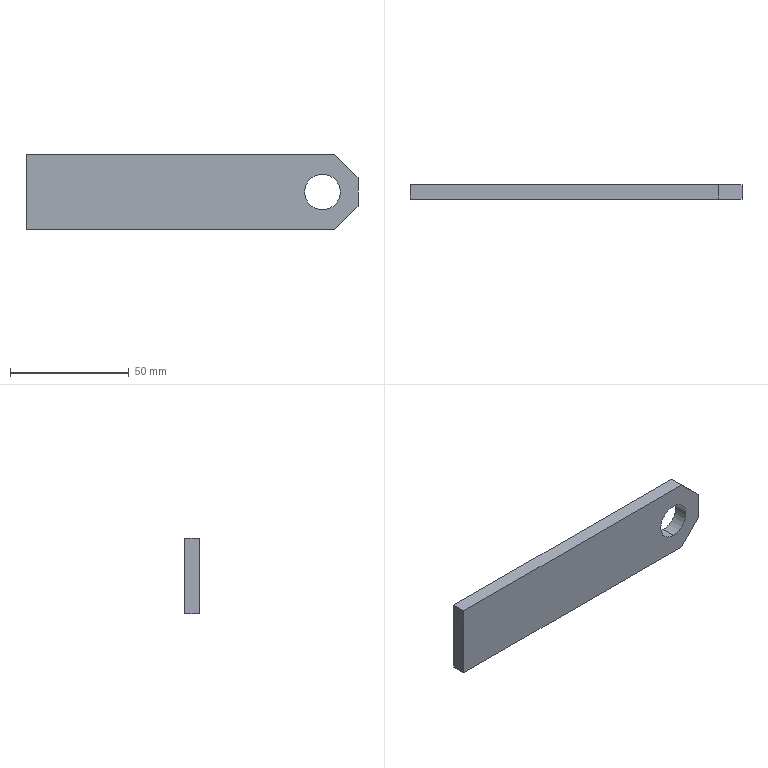Part | SolidWorks | features FlatPattern 1, SMBaseFlange 1, SheetMetal 1 | 1 solid | 10 faces | box 140 x 6 x 32 mm | volume 25220 mm3 | plane 8 | cylinder 2 | commonest cylinder face diameters 15 x2
STEP:
#1=CARTESIAN_POINT('',(125.,-6.,8.5));
#2=VERTEX_POINT('',#1);
#3=CARTESIAN_POINT('',(125.,-6.,23.5));
#4=VERTEX_POINT('',#3);
#5=CARTESIAN_POINT('',(125.,-6.,16.));
#6=DIRECTION('',(0.,1.,0.));
#7=DIRECTION('',(0.,0.,1.));
#8=AXIS2_PLACEMENT_3D('',#5,#6,#7);
#9=CIRCLE('',#8,7.5);
#10=EDGE_CURVE('',#2,#4,#9,.T.);
#11=ORIENTED_EDGE('',*,*,#10,.F.);
#12=CARTESIAN_POINT('',(125.,0.,8.5));
#13=VERTEX_POINT('',#12);
#14=CARTESIAN_POINT('',(125.,-6.,8.5));
#15=DIRECTION('',(0.,1.,0.));
#16=VECTOR('',#15,1000.);
#17=LINE('',#14,#16);
#18=EDGE_CURVE('',#2,#13,#17,.T.);
#19=ORIENTED_EDGE('',*,*,#18,.T.);
#20=CARTESIAN_POINT('',(125.,0.,23.5));
#21=VERTEX_POINT('',#20);
#22=CARTESIAN_POINT('',(125.,0.,16.));
#23=DIRECTION('',(0.,1.,0.));
#24=DIRECTION('',(0.,0.,1.));
#25=AXIS2_PLACEMENT_3D('',#22,#23,#24);
#26=CIRCLE('',#25,7.5);
#27=EDGE_CURVE('',#13,#21,#26,.T.);
#28=ORIENTED_EDGE('',*,*,#27,.T.);
#29=CARTESIAN_POINT('',(125.,-6.,23.5));
#30=DIRECTION('',(0.,1.,0.));
#31=VECTOR('',#30,1000.);
#32=LINE('',#29,#31);
#33=EDGE_CURVE('',#4,#21,#32,.T.);
#34=ORIENTED_EDGE('',*,*,#33,.F.);
#35=EDGE_LOOP('',(#11,#19,#28,#34));
#36=FACE_OUTER_BOUND('',#35,.T.);
#37=CARTESIAN_POINT('',(125.,-6.,16.));
#38=DIRECTION('',(0.,1.,0.));
#39=DIRECTION('',(0.,0.,1.));
#40=AXIS2_PLACEMENT_3D('',#37,#38,#39);
#41=CYLINDRICAL_SURFACE('',#40,7.5);
#42=ADVANCED_FACE('',(#36),#41,.F.);
#43=CARTESIAN_POINT('',(0.,0.,0.));
#44=VERTEX_POINT('',#43);
#45=CARTESIAN_POINT('',(0.,0.,32.));
#46=VERTEX_POINT('',#45);
#47=CARTESIAN_POINT('',(0.,0.,0.));
#48=DIRECTION('',(0.,0.,1.));
#49=VECTOR('',#48,1000.);
#50=LINE('',#47,#49);
#51=EDGE_CURVE('',#44,#46,#50,.T.);
#52=ORIENTED_EDGE('',*,*,#51,.F.);
#53=CARTESIAN_POINT('',(0.,-6.,0.));
#54=VERTEX_POINT('',#53);
#55=CARTESIAN_POINT('',(0.,-6.,0.));
#56=DIRECTION('',(0.,1.,0.));
#57=VECTOR('',#56,1000.);
#58=LINE('',#55,#57);
#59=EDGE_CURVE('',#54,#44,#58,.T.);
#60=ORIENTED_EDGE('',*,*,#59,.F.);
#61=CARTESIAN_POINT('',(0.,-6.,32.));
#62=VERTEX_POINT('',#61);
#63=CARTESIAN_POINT('',(0.,-6.,0.));
#64=DIRECTION('',(0.,0.,1.));
#65=VECTOR('',#64,1000.);
#66=LINE('',#63,#65);
#67=EDGE_CURVE('',#54,#62,#66,.T.);
#68=ORIENTED_EDGE('',*,*,#67,.T.);
#69=CARTESIAN_POINT('',(0.,-6.,32.));
#70=DIRECTION('',(0.,1.,0.));
#71=VECTOR('',#70,1000.);
#72=LINE('',#69,#71);
#73=EDGE_CURVE('',#62,#46,#72,.T.);
#74=ORIENTED_EDGE('',*,*,#73,.T.);
#75=EDGE_LOOP('',(#52,#60,#68,#74));
#76=FACE_OUTER_BOUND('',#75,.T.);
#77=CARTESIAN_POINT('',(0.,-6.,0.));
#78=DIRECTION('',(-1.,0.,0.));
#79=DIRECTION('',(0.,0.,1.));
#80=AXIS2_PLACEMENT_3D('',#77,#78,#79);
#81=PLANE('',#80);
#82=ADVANCED_FACE('',(#76),#81,.T.);
#83=CARTESIAN_POINT('',(130.,0.,0.));
#84=VERTEX_POINT('',#83);
#85=CARTESIAN_POINT('',(0.,0.,0.));
#86=DIRECTION('',(-1.,0.,0.));
#87=VECTOR('',#86,1000.);
#88=LINE('',#85,#87);
#89=EDGE_CURVE('',#84,#44,#88,.T.);
#90=ORIENTED_EDGE('',*,*,#89,.F.);
#91=CARTESIAN_POINT('',(130.,-6.,0.));
#92=VERTEX_POINT('',#91);
#93=CARTESIAN_POINT('',(130.,-6.,0.));
#94=DIRECTION('',(0.,1.,0.));
#95=VECTOR('',#94,1000.);
#96=LINE('',#93,#95);
#97=EDGE_CURVE('',#92,#84,#96,.T.);
#98=ORIENTED_EDGE('',*,*,#97,.F.);
#99=CARTESIAN_POINT('',(0.,-6.,0.));
#100=DIRECTION('',(-1.,0.,0.));
#101=VECTOR('',#100,1000.);
#102=LINE('',#99,#101);
#103=EDGE_CURVE('',#92,#54,#102,.T.);
#104=ORIENTED_EDGE('',*,*,#103,.T.);
#105=ORIENTED_EDGE('',*,*,#59,.T.);
#106=EDGE_LOOP('',(#90,#98,#104,#105));
#107=FACE_OUTER_BOUND('',#106,.T.);
#108=CARTESIAN_POINT('',(0.,-6.,0.));
#109=DIRECTION('',(0.,0.,-1.));
#110=DIRECTION('',(-1.,0.,0.));
#111=AXIS2_PLACEMENT_3D('',#108,#109,#110);
#112=PLANE('',#111);
#113=ADVANCED_FACE('',(#107),#112,.T.);
#114=CARTESIAN_POINT('',(140.,0.,10.));
#115=VERTEX_POINT('',#114);
#116=CARTESIAN_POINT('',(130.,0.,0.));
#117=DIRECTION('',(-0.7071,0.,-0.7071));
#118=VECTOR('',#117,1000.);
#119=LINE('',#116,#118);
#120=EDGE_CURVE('',#115,#84,#119,.T.);
#121=ORIENTED_EDGE('',*,*,#120,.F.);
#122=CARTESIAN_POINT('',(140.,-6.,10.));
#123=VERTEX_POINT('',#122);
#124=CARTESIAN_POINT('',(140.,-6.,10.));
#125=DIRECTION('',(0.,1.,0.));
#126=VECTOR('',#125,1000.);
#127=LINE('',#124,#126);
#128=EDGE_CURVE('',#123,#115,#127,.T.);
#129=ORIENTED_EDGE('',*,*,#128,.F.);
#130=CARTESIAN_POINT('',(130.,-6.,0.));
#131=DIRECTION('',(-0.7071,0.,-0.7071));
#132=VECTOR('',#131,1000.);
#133=LINE('',#130,#132);
#134=EDGE_CURVE('',#123,#92,#133,.T.);
#135=ORIENTED_EDGE('',*,*,#134,.T.);
#136=ORIENTED_EDGE('',*,*,#97,.T.);
#137=EDGE_LOOP('',(#121,#129,#135,#136));
#138=FACE_OUTER_BOUND('',#137,.T.);
#139=CARTESIAN_POINT('',(130.,-6.,0.));
#140=DIRECTION('',(0.7071,0.,-0.7071));
#141=DIRECTION('',(-0.7071,0.,-0.7071));
#142=AXIS2_PLACEMENT_3D('',#139,#140,#141);
#143=PLANE('',#142);
#144=ADVANCED_FACE('',(#138),#143,.T.);
#145=CARTESIAN_POINT('',(140.,0.,22.));
#146=VERTEX_POINT('',#145);
#147=CARTESIAN_POINT('',(140.,0.,10.));
#148=DIRECTION('',(0.,0.,-1.));
#149=VECTOR('',#148,1000.);
#150=LINE('',#147,#149);
#151=EDGE_CURVE('',#146,#115,#150,.T.);
#152=ORIENTED_EDGE('',*,*,#151,.F.);
#153=CARTESIAN_POINT('',(140.,-6.,22.));
#154=VERTEX_POINT('',#153);
#155=CARTESIAN_POINT('',(140.,-6.,22.));
#156=DIRECTION('',(0.,1.,0.));
#157=VECTOR('',#156,1000.);
#158=LINE('',#155,#157);
#159=EDGE_CURVE('',#154,#146,#158,.T.);
#160=ORIENTED_EDGE('',*,*,#159,.F.);
#161=CARTESIAN_POINT('',(140.,-6.,10.));
#162=DIRECTION('',(0.,0.,-1.));
#163=VECTOR('',#162,1000.);
#164=LINE('',#161,#163);
#165=EDGE_CURVE('',#154,#123,#164,.T.);
#166=ORIENTED_EDGE('',*,*,#165,.T.);
#167=ORIENTED_EDGE('',*,*,#128,.T.);
#168=EDGE_LOOP('',(#152,#160,#166,#167));
#169=FACE_OUTER_BOUND('',#168,.T.);
#170=CARTESIAN_POINT('',(140.,-6.,10.));
#171=DIRECTION('',(1.,0.,0.));
#172=DIRECTION('',(0.,0.,-1.));
#173=AXIS2_PLACEMENT_3D('',#170,#171,#172);
#174=PLANE('',#173);
#175=ADVANCED_FACE('',(#169),#174,.T.);
#176=CARTESIAN_POINT('',(130.,0.,32.));
#177=VERTEX_POINT('',#176);
#178=CARTESIAN_POINT('',(130.,0.,32.));
#179=DIRECTION('',(0.7071,0.,-0.7071));
#180=VECTOR('',#179,1000.);
#181=LINE('',#178,#180);
#182=EDGE_CURVE('',#177,#146,#181,.T.);
#183=ORIENTED_EDGE('',*,*,#182,.F.);
#184=CARTESIAN_POINT('',(130.,-6.,32.));
#185=VERTEX_POINT('',#184);
#186=CARTESIAN_POINT('',(130.,-6.,32.));
#187=DIRECTION('',(0.,1.,0.));
#188=VECTOR('',#187,1000.);
#189=LINE('',#186,#188);
#190=EDGE_CURVE('',#185,#177,#189,.T.);
#191=ORIENTED_EDGE('',*,*,#190,.F.);
#192=CARTESIAN_POINT('',(130.,-6.,32.));
#193=DIRECTION('',(0.7071,0.,-0.7071));
#194=VECTOR('',#193,1000.);
#195=LINE('',#192,#194);
#196=EDGE_CURVE('',#185,#154,#195,.T.);
#197=ORIENTED_EDGE('',*,*,#196,.T.);
#198=ORIENTED_EDGE('',*,*,#159,.T.);
#199=EDGE_LOOP('',(#183,#191,#197,#198));
#200=FACE_OUTER_BOUND('',#199,.T.);
#201=CARTESIAN_POINT('',(130.,-6.,32.));
#202=DIRECTION('',(0.7071,0.,0.7071));
#203=DIRECTION('',(0.7071,0.,-0.7071));
#204=AXIS2_PLACEMENT_3D('',#201,#202,#203);
#205=PLANE('',#204);
#206=ADVANCED_FACE('',(#200),#205,.T.);
#207=CARTESIAN_POINT('',(0.,0.,32.));
#208=DIRECTION('',(1.,0.,0.));
#209=VECTOR('',#208,1000.);
#210=LINE('',#207,#209);
#211=EDGE_CURVE('',#46,#177,#210,.T.);
#212=ORIENTED_EDGE('',*,*,#211,.F.);
#213=ORIENTED_EDGE('',*,*,#73,.F.);
#214=CARTESIAN_POINT('',(0.,-6.,32.));
#215=DIRECTION('',(1.,0.,0.));
#216=VECTOR('',#215,1000.);
#217=LINE('',#214,#216);
#218=EDGE_CURVE('',#62,#185,#217,.T.);
#219=ORIENTED_EDGE('',*,*,#218,.T.);
#220=ORIENTED_EDGE('',*,*,#190,.T.);
#221=EDGE_LOOP('',(#212,#213,#219,#220));
#222=FACE_OUTER_BOUND('',#221,.T.);
#223=CARTESIAN_POINT('',(0.,-6.,32.));
#224=DIRECTION('',(0.,0.,1.));
#225=DIRECTION('',(1.,0.,0.));
#226=AXIS2_PLACEMENT_3D('',#223,#224,#225);
#227=PLANE('',#226);
#228=ADVANCED_FACE('',(#222),#227,.T.);
#229=CARTESIAN_POINT('',(125.,-6.,16.));
#230=DIRECTION('',(0.,1.,0.));
#231=DIRECTION('',(0.,0.,1.));
#232=AXIS2_PLACEMENT_3D('',#229,#230,#231);
#233=CIRCLE('',#232,7.5);
#234=EDGE_CURVE('',#4,#2,#233,.T.);
#235=ORIENTED_EDGE('',*,*,#234,.T.);
#236=ORIENTED_EDGE('',*,*,#10,.T.);
#237=EDGE_LOOP('',(#235,#236));
#238=FACE_BOUND('',#237,.T.);
#239=ORIENTED_EDGE('',*,*,#67,.F.);
#240=ORIENTED_EDGE('',*,*,#103,.F.);
#241=ORIENTED_EDGE('',*,*,#134,.F.);
#242=ORIENTED_EDGE('',*,*,#165,.F.);
#243=ORIENTED_EDGE('',*,*,#196,.F.);
#244=ORIENTED_EDGE('',*,*,#218,.F.);
#245=EDGE_LOOP('',(#239,#240,#241,#242,#243,#244));
#246=FACE_OUTER_BOUND('',#245,.T.);
#247=CARTESIAN_POINT('',(0.,-6.,0.));
#248=DIRECTION('',(0.,1.,0.));
#249=DIRECTION('',(0.,0.,1.));
#250=AXIS2_PLACEMENT_3D('',#247,#248,#249);
#251=PLANE('',#250);
#252=ADVANCED_FACE('',(#238,#246),#251,.F.);
#253=CARTESIAN_POINT('',(125.,0.,16.));
#254=DIRECTION('',(0.,1.,0.));
#255=DIRECTION('',(0.,0.,1.));
#256=AXIS2_PLACEMENT_3D('',#253,#254,#255);
#257=CIRCLE('',#256,7.5);
#258=EDGE_CURVE('',#21,#13,#257,.T.);
#259=ORIENTED_EDGE('',*,*,#258,.F.);
#260=ORIENTED_EDGE('',*,*,#27,.F.);
#261=EDGE_LOOP('',(#259,#260));
#262=FACE_BOUND('',#261,.T.);
#263=ORIENTED_EDGE('',*,*,#51,.T.);
#264=ORIENTED_EDGE('',*,*,#211,.T.);
#265=ORIENTED_EDGE('',*,*,#182,.T.);
#266=ORIENTED_EDGE('',*,*,#151,.T.);
#267=ORIENTED_EDGE('',*,*,#120,.T.);
#268=ORIENTED_EDGE('',*,*,#89,.T.);
#269=EDGE_LOOP('',(#263,#264,#265,#266,#267,#268));
#270=FACE_OUTER_BOUND('',#269,.T.);
#271=CARTESIAN_POINT('',(0.,0.,0.));
#272=DIRECTION('',(0.,1.,0.));
#273=DIRECTION('',(0.,0.,1.));
#274=AXIS2_PLACEMENT_3D('',#271,#272,#273);
#275=PLANE('',#274);
#276=ADVANCED_FACE('',(#262,#270),#275,.T.);
#277=ORIENTED_EDGE('',*,*,#18,.F.);
#278=ORIENTED_EDGE('',*,*,#234,.F.);
#279=ORIENTED_EDGE('',*,*,#33,.T.);
#280=ORIENTED_EDGE('',*,*,#258,.T.);
#281=EDGE_LOOP('',(#277,#278,#279,#280));
#282=FACE_OUTER_BOUND('',#281,.T.);
#283=CARTESIAN_POINT('',(125.,-6.,16.));
#284=DIRECTION('',(0.,1.,0.));
#285=DIRECTION('',(0.,0.,1.));
#286=AXIS2_PLACEMENT_3D('',#283,#284,#285);
#287=CYLINDRICAL_SURFACE('',#286,7.5);
#288=ADVANCED_FACE('',(#282),#287,.F.);
#289=CLOSED_SHELL('',(#42,#82,#113,#144,#175,#206,#228,#252,#276,#288));
#290=MANIFOLD_SOLID_BREP('',#289);
#291=CARTESIAN_POINT('',(0.,0.,0.));
#292=DIRECTION('',(0.,0.,1.));
#293=DIRECTION('',(1.,0.,0.));
#294=AXIS2_PLACEMENT_3D('',#291,#292,#293);
#295=(LENGTH_UNIT()NAMED_UNIT(*)SI_UNIT(.MILLI.,.METRE.));
#296=UNCERTAINTY_MEASURE_WITH_UNIT(LENGTH_MEASURE(0.00001),#295,'','');
#297=(NAMED_UNIT(*)PLANE_ANGLE_UNIT()SI_UNIT($,.RADIAN.));
#298=(NAMED_UNIT(*)SI_UNIT($,.STERADIAN.)SOLID_ANGLE_UNIT());
#299=(GEOMETRIC_REPRESENTATION_CONTEXT(3)GLOBAL_UNCERTAINTY_ASSIGNED_CONTEXT((#296))GLOBAL_UNIT_ASSIGNED_CONTEXT((#295,#297,#298))REPRESENTATION_CONTEXT('',''));
#300=ADVANCED_BREP_SHAPE_REPRESENTATION('',(#290,#294),#299);